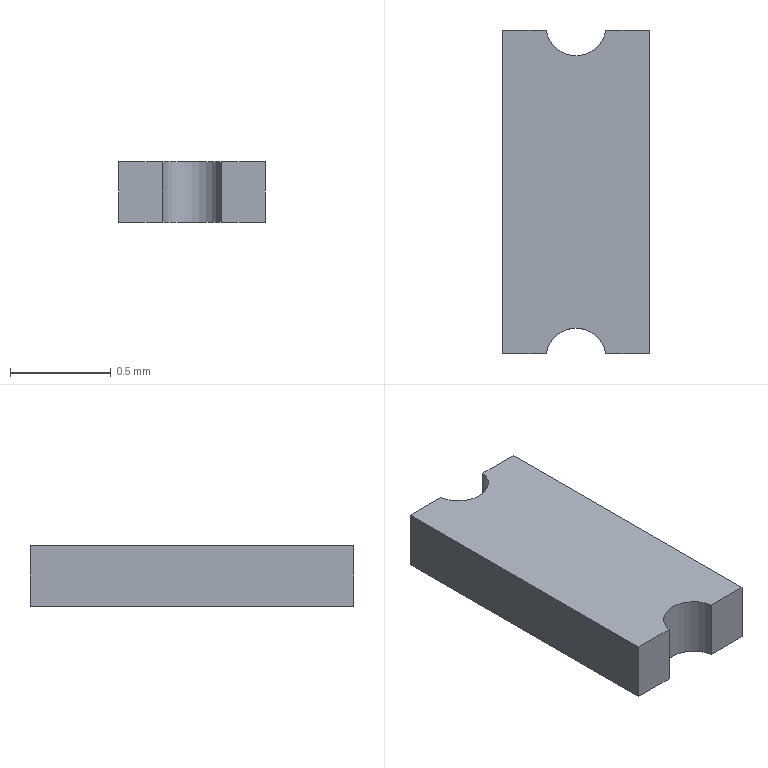Part | STEP file | RJ-USIO-V1_2-220411_160 | 1 solid | 10 faces | box 0.725 x 1.6 x 0.3 mm | volume 0.3313 mm3 | plane 8 | cylinder 2 | commonest cylinder face diameters 0.3 x2
STEP:
#1=CARTESIAN_POINT('',(0.,0.,0.));
#2=DIRECTION('',(0.,0.,1.));
#3=DIRECTION('',(1.,0.,0.));
#4=AXIS2_PLACEMENT_3D('',#1,#2,#3);
#5=CARTESIAN_POINT('',(60.137,66.1,0.3298));
#6=VERTEX_POINT('',#5);
#7=CARTESIAN_POINT('',(60.137,67.7,0.3298));
#8=VERTEX_POINT('',#7);
#9=CARTESIAN_POINT('',(60.137,66.1,0.3298));
#10=DIRECTION('',(-0.000000175,1.,0.));
#11=VECTOR('',#10,1.);
#12=LINE('',#9,#11);
#13=CARTESIAN_POINT('',(60.5,66.9,0.3298));
#14=DIRECTION('',(0.,0.,1.));
#15=DIRECTION('',(-1.,-0.000000175,0.));
#16=AXIS2_PLACEMENT_3D('',#13,#14,#15);
#17=PLANE('',#16);
#18=CARTESIAN_POINT('',(0.3625,0.8));
#19=DIRECTION('',(0.,-1.));
#20=VECTOR('',#19,1.);
#21=LINE('',#18,#20);
#22=(GEOMETRIC_REPRESENTATION_CONTEXT(2)PARAMETRIC_REPRESENTATION_CONTEXT()REPRESENTATION_CONTEXT('',''));
#23=DEFINITIONAL_REPRESENTATION('',(#21),#22);
#24=PCURVE('',#17,#23);
#25=CARTESIAN_POINT('',(60.137,67.7,0.02977));
#26=DIRECTION('',(-1.,-0.000000175,0.));
#27=DIRECTION('',(-0.000000175,1.,0.));
#28=AXIS2_PLACEMENT_3D('',#25,#26,#27);
#29=PLANE('',#28);
#30=CARTESIAN_POINT('',(-1.6,-0.3));
#31=DIRECTION('',(1.,0.));
#32=VECTOR('',#31,1.);
#33=LINE('',#30,#32);
#34=(GEOMETRIC_REPRESENTATION_CONTEXT(2)PARAMETRIC_REPRESENTATION_CONTEXT()REPRESENTATION_CONTEXT('',''));
#35=DEFINITIONAL_REPRESENTATION('',(#33),#34);
#36=PCURVE('',#29,#35);
#37=SURFACE_CURVE('',#12,(#24,#36),.PCURVE_S1.);
#38=EDGE_CURVE('',#6,#8,#37,.T.);
#39=ORIENTED_EDGE('',*,*,#38,.T.);
#40=CARTESIAN_POINT('',(60.352,67.7,0.3298));
#41=VERTEX_POINT('',#40);
#42=CARTESIAN_POINT('',(60.137,67.7,0.3298));
#43=DIRECTION('',(1.,0.000000175,0.));
#44=VECTOR('',#43,1.);
#45=LINE('',#42,#44);
#46=CARTESIAN_POINT('',(0.3625,-0.8));
#47=DIRECTION('',(-1.,0.));
#48=VECTOR('',#47,1.);
#49=LINE('',#46,#48);
#50=(GEOMETRIC_REPRESENTATION_CONTEXT(2)PARAMETRIC_REPRESENTATION_CONTEXT()REPRESENTATION_CONTEXT('',''));
#51=DEFINITIONAL_REPRESENTATION('',(#49),#50);
#52=PCURVE('',#17,#51);
#53=CARTESIAN_POINT('',(60.862,67.7,0.02977));
#54=DIRECTION('',(-0.000000175,1.,0.));
#55=DIRECTION('',(1.,0.000000175,0.));
#56=AXIS2_PLACEMENT_3D('',#53,#54,#55);
#57=PLANE('',#56);
#58=CARTESIAN_POINT('',(-0.725,-0.3));
#59=DIRECTION('',(1.,0.));
#60=VECTOR('',#59,1.);
#61=LINE('',#58,#60);
#62=(GEOMETRIC_REPRESENTATION_CONTEXT(2)PARAMETRIC_REPRESENTATION_CONTEXT()REPRESENTATION_CONTEXT('',''));
#63=DEFINITIONAL_REPRESENTATION('',(#61),#62);
#64=PCURVE('',#57,#63);
#65=SURFACE_CURVE('',#45,(#52,#64),.PCURVE_S1.);
#66=EDGE_CURVE('',#8,#41,#65,.T.);
#67=ORIENTED_EDGE('',*,*,#66,.T.);
#68=CARTESIAN_POINT('',(60.648,67.7,0.3298));
#69=VERTEX_POINT('',#68);
#70=CARTESIAN_POINT('',(60.5,67.725,0.3298));
#71=DIRECTION('',(0.,0.,-1.));
#72=DIRECTION('',(0.986,-0.1667,0.));
#73=AXIS2_PLACEMENT_3D('',#70,#71,#72);
#74=CIRCLE('',#73,0.15);
#75=CARTESIAN_POINT('',(-0.1479,-0.8));
#76=CARTESIAN_POINT('',(-0.1046,-0.5438));
#77=CARTESIAN_POINT('',(0.0956,-0.7094));
#78=CARTESIAN_POINT('',(0.2958,-0.875));
#79=CARTESIAN_POINT('',(0.0523,-0.9656));
#80=CARTESIAN_POINT('',(-0.1912,-1.056));
#81=CARTESIAN_POINT('',(-0.1479,-0.8));
#82=(BOUNDED_CURVE()B_SPLINE_CURVE(2,(#75,#76,#77,#78,#79,#80,#81),.UNSPECIFIED.,.T.,.F.)B_SPLINE_CURVE_WITH_KNOTS((1,2,2,2,2,1),(-2.094,0.,2.094,4.189,6.283,8.378),.UNSPECIFIED.)CURVE()GEOMETRIC_REPRESENTATION_ITEM()RATIONAL_B_SPLINE_CURVE((1.,0.5,1.,0.5,1.,0.5,1.))REPRESENTATION_ITEM(''));
#83=(GEOMETRIC_REPRESENTATION_CONTEXT(2)PARAMETRIC_REPRESENTATION_CONTEXT()REPRESENTATION_CONTEXT('',''));
#84=DEFINITIONAL_REPRESENTATION('',(#82),#83);
#85=PCURVE('',#17,#84);
#86=CARTESIAN_POINT('',(60.5,67.725,-0.2214));
#87=DIRECTION('',(0.,0.,-1.));
#88=DIRECTION('',(1.,0.000000175,0.));
#89=AXIS2_PLACEMENT_3D('',#86,#87,#88);
#90=CYLINDRICAL_SURFACE('',#89,0.15);
#91=CARTESIAN_POINT('',(0.1674,-0.5512));
#92=DIRECTION('',(1.,0.));
#93=VECTOR('',#92,1.);
#94=LINE('',#91,#93);
#95=(GEOMETRIC_REPRESENTATION_CONTEXT(2)PARAMETRIC_REPRESENTATION_CONTEXT()REPRESENTATION_CONTEXT('',''));
#96=DEFINITIONAL_REPRESENTATION('',(#94),#95);
#97=PCURVE('',#90,#96);
#98=SURFACE_CURVE('',#74,(#85,#97),.PCURVE_S1.);
#99=EDGE_CURVE('',#69,#41,#98,.T.);
#100=ORIENTED_EDGE('',*,*,#99,.F.);
#101=CARTESIAN_POINT('',(60.862,67.7,0.3298));
#102=VERTEX_POINT('',#101);
#103=CARTESIAN_POINT('',(60.648,67.7,0.3298));
#104=DIRECTION('',(1.,0.000000175,0.));
#105=VECTOR('',#104,1.);
#106=LINE('',#103,#105);
#107=CARTESIAN_POINT('',(-0.1479,-0.8));
#108=DIRECTION('',(-1.,0.));
#109=VECTOR('',#108,1.);
#110=LINE('',#107,#109);
#111=(GEOMETRIC_REPRESENTATION_CONTEXT(2)PARAMETRIC_REPRESENTATION_CONTEXT()REPRESENTATION_CONTEXT('',''));
#112=DEFINITIONAL_REPRESENTATION('',(#110),#111);
#113=PCURVE('',#17,#112);
#114=CARTESIAN_POINT('',(60.862,67.7,0.02977));
#115=DIRECTION('',(-0.000000175,1.,0.));
#116=DIRECTION('',(1.,0.000000175,0.));
#117=AXIS2_PLACEMENT_3D('',#114,#115,#116);
#118=PLANE('',#117);
#119=CARTESIAN_POINT('',(-0.2146,-0.3));
#120=DIRECTION('',(1.,0.));
#121=VECTOR('',#120,1.);
#122=LINE('',#119,#121);
#123=(GEOMETRIC_REPRESENTATION_CONTEXT(2)PARAMETRIC_REPRESENTATION_CONTEXT()REPRESENTATION_CONTEXT('',''));
#124=DEFINITIONAL_REPRESENTATION('',(#122),#123);
#125=PCURVE('',#118,#124);
#126=SURFACE_CURVE('',#106,(#113,#125),.PCURVE_S1.);
#127=EDGE_CURVE('',#69,#102,#126,.T.);
#128=ORIENTED_EDGE('',*,*,#127,.T.);
#129=CARTESIAN_POINT('',(60.862,66.1,0.3298));
#130=VERTEX_POINT('',#129);
#131=CARTESIAN_POINT('',(60.862,67.7,0.3298));
#132=DIRECTION('',(0.000000175,-1.,0.));
#133=VECTOR('',#132,1.);
#134=LINE('',#131,#133);
#135=CARTESIAN_POINT('',(-0.3625,-0.8));
#136=DIRECTION('',(0.,1.));
#137=VECTOR('',#136,1.);
#138=LINE('',#135,#137);
#139=(GEOMETRIC_REPRESENTATION_CONTEXT(2)PARAMETRIC_REPRESENTATION_CONTEXT()REPRESENTATION_CONTEXT('',''));
#140=DEFINITIONAL_REPRESENTATION('',(#138),#139);
#141=PCURVE('',#17,#140);
#142=CARTESIAN_POINT('',(60.862,66.1,0.02977));
#143=DIRECTION('',(1.,0.000000175,0.));
#144=DIRECTION('',(0.000000175,-1.,0.));
#145=AXIS2_PLACEMENT_3D('',#142,#143,#144);
#146=PLANE('',#145);
#147=CARTESIAN_POINT('',(-1.6,-0.3));
#148=DIRECTION('',(1.,0.));
#149=VECTOR('',#148,1.);
#150=LINE('',#147,#149);
#151=(GEOMETRIC_REPRESENTATION_CONTEXT(2)PARAMETRIC_REPRESENTATION_CONTEXT()REPRESENTATION_CONTEXT('',''));
#152=DEFINITIONAL_REPRESENTATION('',(#150),#151);
#153=PCURVE('',#146,#152);
#154=SURFACE_CURVE('',#134,(#141,#153),.PCURVE_S1.);
#155=EDGE_CURVE('',#102,#130,#154,.T.);
#156=ORIENTED_EDGE('',*,*,#155,.T.);
#157=CARTESIAN_POINT('',(60.648,66.1,0.3298));
#158=VERTEX_POINT('',#157);
#159=CARTESIAN_POINT('',(60.862,66.1,0.3298));
#160=DIRECTION('',(-1.,-0.000000175,0.));
#161=VECTOR('',#160,1.);
#162=LINE('',#159,#161);
#163=CARTESIAN_POINT('',(-0.3625,0.8));
#164=DIRECTION('',(1.,0.));
#165=VECTOR('',#164,1.);
#166=LINE('',#163,#165);
#167=(GEOMETRIC_REPRESENTATION_CONTEXT(2)PARAMETRIC_REPRESENTATION_CONTEXT()REPRESENTATION_CONTEXT('',''));
#168=DEFINITIONAL_REPRESENTATION('',(#166),#167);
#169=PCURVE('',#17,#168);
#170=CARTESIAN_POINT('',(60.862,66.1,0.02977));
#171=DIRECTION('',(0.000000175,-1.,0.));
#172=DIRECTION('',(-1.,-0.000000175,0.));
#173=AXIS2_PLACEMENT_3D('',#170,#171,#172);
#174=PLANE('',#173);
#175=CARTESIAN_POINT('',(0.,-0.3));
#176=DIRECTION('',(1.,0.));
#177=VECTOR('',#176,1.);
#178=LINE('',#175,#177);
#179=(GEOMETRIC_REPRESENTATION_CONTEXT(2)PARAMETRIC_REPRESENTATION_CONTEXT()REPRESENTATION_CONTEXT('',''));
#180=DEFINITIONAL_REPRESENTATION('',(#178),#179);
#181=PCURVE('',#174,#180);
#182=SURFACE_CURVE('',#162,(#169,#181),.PCURVE_S1.);
#183=EDGE_CURVE('',#130,#158,#182,.T.);
#184=ORIENTED_EDGE('',*,*,#183,.T.);
#185=CARTESIAN_POINT('',(60.352,66.1,0.3298));
#186=VERTEX_POINT('',#185);
#187=CARTESIAN_POINT('',(60.5,66.075,0.3298));
#188=DIRECTION('',(0.,0.,-1.));
#189=DIRECTION('',(-0.986,0.1667,0.));
#190=AXIS2_PLACEMENT_3D('',#187,#188,#189);
#191=CIRCLE('',#190,0.15);
#192=CARTESIAN_POINT('',(0.1479,0.8));
#193=CARTESIAN_POINT('',(0.1046,0.5438));
#194=CARTESIAN_POINT('',(-0.0956,0.7094));
#195=CARTESIAN_POINT('',(-0.2958,0.875));
#196=CARTESIAN_POINT('',(-0.0523,0.9656));
#197=CARTESIAN_POINT('',(0.1912,1.056));
#198=CARTESIAN_POINT('',(0.1479,0.8));
#199=(BOUNDED_CURVE()B_SPLINE_CURVE(2,(#192,#193,#194,#195,#196,#197,#198),.UNSPECIFIED.,.T.,.F.)B_SPLINE_CURVE_WITH_KNOTS((1,2,2,2,2,1),(-2.094,0.,2.094,4.189,6.283,8.378),.UNSPECIFIED.)CURVE()GEOMETRIC_REPRESENTATION_ITEM()RATIONAL_B_SPLINE_CURVE((1.,0.5,1.,0.5,1.,0.5,1.))REPRESENTATION_ITEM(''));
#200=(GEOMETRIC_REPRESENTATION_CONTEXT(2)PARAMETRIC_REPRESENTATION_CONTEXT()REPRESENTATION_CONTEXT('',''));
#201=DEFINITIONAL_REPRESENTATION('',(#199),#200);
#202=PCURVE('',#17,#201);
#203=CARTESIAN_POINT('',(60.5,66.075,-0.2214));
#204=DIRECTION('',(0.,0.,1.));
#205=DIRECTION('',(-1.,-0.000000175,0.));
#206=AXIS2_PLACEMENT_3D('',#203,#204,#205);
#207=CYLINDRICAL_SURFACE('',#206,0.15);
#208=CARTESIAN_POINT('',(6.116,0.5512));
#209=DIRECTION('',(-1.,0.));
#210=VECTOR('',#209,1.);
#211=LINE('',#208,#210);
#212=(GEOMETRIC_REPRESENTATION_CONTEXT(2)PARAMETRIC_REPRESENTATION_CONTEXT()REPRESENTATION_CONTEXT('',''));
#213=DEFINITIONAL_REPRESENTATION('',(#211),#212);
#214=PCURVE('',#207,#213);
#215=SURFACE_CURVE('',#191,(#202,#214),.PCURVE_S1.);
#216=EDGE_CURVE('',#186,#158,#215,.T.);
#217=ORIENTED_EDGE('',*,*,#216,.F.);
#218=CARTESIAN_POINT('',(60.352,66.1,0.3298));
#219=DIRECTION('',(-1.,-0.000000175,0.));
#220=VECTOR('',#219,1.);
#221=LINE('',#218,#220);
#222=CARTESIAN_POINT('',(0.1479,0.8));
#223=DIRECTION('',(1.,0.));
#224=VECTOR('',#223,1.);
#225=LINE('',#222,#224);
#226=(GEOMETRIC_REPRESENTATION_CONTEXT(2)PARAMETRIC_REPRESENTATION_CONTEXT()REPRESENTATION_CONTEXT('',''));
#227=DEFINITIONAL_REPRESENTATION('',(#225),#226);
#228=PCURVE('',#17,#227);
#229=CARTESIAN_POINT('',(60.862,66.1,0.02977));
#230=DIRECTION('',(0.000000175,-1.,0.));
#231=DIRECTION('',(-1.,-0.000000175,0.));
#232=AXIS2_PLACEMENT_3D('',#229,#230,#231);
#233=PLANE('',#232);
#234=CARTESIAN_POINT('',(0.5104,-0.3));
#235=DIRECTION('',(1.,0.));
#236=VECTOR('',#235,1.);
#237=LINE('',#234,#236);
#238=(GEOMETRIC_REPRESENTATION_CONTEXT(2)PARAMETRIC_REPRESENTATION_CONTEXT()REPRESENTATION_CONTEXT('',''));
#239=DEFINITIONAL_REPRESENTATION('',(#237),#238);
#240=PCURVE('',#233,#239);
#241=SURFACE_CURVE('',#221,(#228,#240),.PCURVE_S1.);
#242=EDGE_CURVE('',#186,#6,#241,.T.);
#243=ORIENTED_EDGE('',*,*,#242,.T.);
#244=EDGE_LOOP('',(#39,#67,#100,#128,#156,#184,#217,#243));
#245=FACE_BOUND('',#244,.F.);
#246=ADVANCED_FACE('',(#245),#17,.T.);
#247=ORIENTED_EDGE('',*,*,#38,.F.);
#248=CARTESIAN_POINT('',(60.137,66.1,0.02977));
#249=VERTEX_POINT('',#248);
#250=CARTESIAN_POINT('',(60.137,66.1,0.02977));
#251=DIRECTION('',(0.,0.,1.));
#252=VECTOR('',#251,1.);
#253=LINE('',#250,#252);
#254=CARTESIAN_POINT('',(-1.6,0.));
#255=DIRECTION('',(0.,-1.));
#256=VECTOR('',#255,1.);
#257=LINE('',#254,#256);
#258=(GEOMETRIC_REPRESENTATION_CONTEXT(2)PARAMETRIC_REPRESENTATION_CONTEXT()REPRESENTATION_CONTEXT('',''));
#259=DEFINITIONAL_REPRESENTATION('',(#257),#258);
#260=PCURVE('',#29,#259);
#261=CARTESIAN_POINT('',(0.725,0.));
#262=DIRECTION('',(0.,-1.));
#263=VECTOR('',#262,1.);
#264=LINE('',#261,#263);
#265=(GEOMETRIC_REPRESENTATION_CONTEXT(2)PARAMETRIC_REPRESENTATION_CONTEXT()REPRESENTATION_CONTEXT('',''));
#266=DEFINITIONAL_REPRESENTATION('',(#264),#265);
#267=PCURVE('',#233,#266);
#268=SURFACE_CURVE('',#253,(#260,#267),.PCURVE_S1.);
#269=EDGE_CURVE('',#249,#6,#268,.T.);
#270=ORIENTED_EDGE('',*,*,#269,.F.);
#271=CARTESIAN_POINT('',(60.137,67.7,0.02977));
#272=VERTEX_POINT('',#271);
#273=CARTESIAN_POINT('',(60.137,66.1,0.02977));
#274=DIRECTION('',(-0.000000175,1.,0.));
#275=VECTOR('',#274,1.);
#276=LINE('',#273,#275);
#277=CARTESIAN_POINT('',(-1.6,0.));
#278=DIRECTION('',(1.,0.));
#279=VECTOR('',#278,1.);
#280=LINE('',#277,#279);
#281=(GEOMETRIC_REPRESENTATION_CONTEXT(2)PARAMETRIC_REPRESENTATION_CONTEXT()REPRESENTATION_CONTEXT('',''));
#282=DEFINITIONAL_REPRESENTATION('',(#280),#281);
#283=PCURVE('',#29,#282);
#284=CARTESIAN_POINT('',(60.5,66.9,0.02977));
#285=DIRECTION('',(0.,0.,1.));
#286=DIRECTION('',(-1.,-0.000000175,0.));
#287=AXIS2_PLACEMENT_3D('',#284,#285,#286);
#288=PLANE('',#287);
#289=CARTESIAN_POINT('',(0.3625,0.8));
#290=DIRECTION('',(0.,-1.));
#291=VECTOR('',#290,1.);
#292=LINE('',#289,#291);
#293=(GEOMETRIC_REPRESENTATION_CONTEXT(2)PARAMETRIC_REPRESENTATION_CONTEXT()REPRESENTATION_CONTEXT('',''));
#294=DEFINITIONAL_REPRESENTATION('',(#292),#293);
#295=PCURVE('',#288,#294);
#296=SURFACE_CURVE('',#276,(#283,#295),.PCURVE_S1.);
#297=EDGE_CURVE('',#249,#272,#296,.T.);
#298=ORIENTED_EDGE('',*,*,#297,.T.);
#299=CARTESIAN_POINT('',(60.137,67.7,0.02977));
#300=DIRECTION('',(0.,0.,1.));
#301=VECTOR('',#300,1.);
#302=LINE('',#299,#301);
#303=CARTESIAN_POINT('',(0.,0.));
#304=DIRECTION('',(0.,-1.));
#305=VECTOR('',#304,1.);
#306=LINE('',#303,#305);
#307=(GEOMETRIC_REPRESENTATION_CONTEXT(2)PARAMETRIC_REPRESENTATION_CONTEXT()REPRESENTATION_CONTEXT('',''));
#308=DEFINITIONAL_REPRESENTATION('',(#306),#307);
#309=PCURVE('',#29,#308);
#310=CARTESIAN_POINT('',(-0.725,0.));
#311=DIRECTION('',(0.,-1.));
#312=VECTOR('',#311,1.);
#313=LINE('',#310,#312);
#314=(GEOMETRIC_REPRESENTATION_CONTEXT(2)PARAMETRIC_REPRESENTATION_CONTEXT()REPRESENTATION_CONTEXT('',''));
#315=DEFINITIONAL_REPRESENTATION('',(#313),#314);
#316=PCURVE('',#57,#315);
#317=SURFACE_CURVE('',#302,(#309,#316),.PCURVE_S1.);
#318=EDGE_CURVE('',#272,#8,#317,.T.);
#319=ORIENTED_EDGE('',*,*,#318,.T.);
#320=EDGE_LOOP('',(#247,#270,#298,#319));
#321=FACE_BOUND('',#320,.F.);
#322=ADVANCED_FACE('',(#321),#29,.T.);
#323=CARTESIAN_POINT('',(60.352,66.1,0.02977));
#324=VERTEX_POINT('',#323);
#325=CARTESIAN_POINT('',(60.352,66.1,0.3298));
#326=DIRECTION('',(0.,0.,-1.));
#327=VECTOR('',#326,1.);
#328=LINE('',#325,#327);
#329=CARTESIAN_POINT('',(0.5104,-0.3));
#330=DIRECTION('',(0.,1.));
#331=VECTOR('',#330,1.);
#332=LINE('',#329,#331);
#333=(GEOMETRIC_REPRESENTATION_CONTEXT(2)PARAMETRIC_REPRESENTATION_CONTEXT()REPRESENTATION_CONTEXT('',''));
#334=DEFINITIONAL_REPRESENTATION('',(#332),#333);
#335=PCURVE('',#233,#334);
#336=CARTESIAN_POINT('',(6.116,0.5512));
#337=DIRECTION('',(0.,-1.));
#338=VECTOR('',#337,1.);
#339=LINE('',#336,#338);
#340=(GEOMETRIC_REPRESENTATION_CONTEXT(2)PARAMETRIC_REPRESENTATION_CONTEXT()REPRESENTATION_CONTEXT('',''));
#341=DEFINITIONAL_REPRESENTATION('',(#339),#340);
#342=PCURVE('',#207,#341);
#343=SURFACE_CURVE('',#328,(#335,#342),.PCURVE_S1.);
#344=EDGE_CURVE('',#186,#324,#343,.T.);
#345=ORIENTED_EDGE('',*,*,#344,.T.);
#346=CARTESIAN_POINT('',(60.352,66.1,0.02977));
#347=DIRECTION('',(-1.,-0.000000175,0.));
#348=VECTOR('',#347,1.);
#349=LINE('',#346,#348);
#350=CARTESIAN_POINT('',(0.5104,0.));
#351=DIRECTION('',(1.,0.));
#352=VECTOR('',#351,1.);
#353=LINE('',#350,#352);
#354=(GEOMETRIC_REPRESENTATION_CONTEXT(2)PARAMETRIC_REPRESENTATION_CONTEXT()REPRESENTATION_CONTEXT('',''));
#355=DEFINITIONAL_REPRESENTATION('',(#353),#354);
#356=PCURVE('',#233,#355);
#357=CARTESIAN_POINT('',(0.1479,0.8));
#358=DIRECTION('',(1.,0.));
#359=VECTOR('',#358,1.);
#360=LINE('',#357,#359);
#361=(GEOMETRIC_REPRESENTATION_CONTEXT(2)PARAMETRIC_REPRESENTATION_CONTEXT()REPRESENTATION_CONTEXT('',''));
#362=DEFINITIONAL_REPRESENTATION('',(#360),#361);
#363=PCURVE('',#288,#362);
#364=SURFACE_CURVE('',#349,(#356,#363),.PCURVE_S1.);
#365=EDGE_CURVE('',#324,#249,#364,.T.);
#366=ORIENTED_EDGE('',*,*,#365,.T.);
#367=ORIENTED_EDGE('',*,*,#269,.T.);
#368=ORIENTED_EDGE('',*,*,#242,.F.);
#369=EDGE_LOOP('',(#345,#366,#367,#368));
#370=FACE_BOUND('',#369,.F.);
#371=ADVANCED_FACE('',(#370),#233,.T.);
#372=CARTESIAN_POINT('',(60.648,66.1,0.02977));
#373=VERTEX_POINT('',#372);
#374=CARTESIAN_POINT('',(60.5,66.075,0.02977));
#375=DIRECTION('',(0.,0.,1.));
#376=DIRECTION('',(0.986,0.1667,0.));
#377=AXIS2_PLACEMENT_3D('',#374,#375,#376);
#378=CIRCLE('',#377,0.15);
#379=CARTESIAN_POINT('',(3.309,0.2512));
#380=DIRECTION('',(1.,0.));
#381=VECTOR('',#380,1.);
#382=LINE('',#379,#381);
#383=(GEOMETRIC_REPRESENTATION_CONTEXT(2)PARAMETRIC_REPRESENTATION_CONTEXT()REPRESENTATION_CONTEXT('',''));
#384=DEFINITIONAL_REPRESENTATION('',(#382),#383);
#385=PCURVE('',#207,#384);
#386=CARTESIAN_POINT('',(0.,0.825));
#387=DIRECTION('',(-0.986,-0.1667));
#388=AXIS2_PLACEMENT_2D('',#386,#387);
#389=CIRCLE('',#388,0.15);
#390=(GEOMETRIC_REPRESENTATION_CONTEXT(2)PARAMETRIC_REPRESENTATION_CONTEXT()REPRESENTATION_CONTEXT('',''));
#391=DEFINITIONAL_REPRESENTATION('',(#389),#390);
#392=PCURVE('',#288,#391);
#393=SURFACE_CURVE('',#378,(#385,#392),.PCURVE_S1.);
#394=EDGE_CURVE('',#373,#324,#393,.T.);
#395=ORIENTED_EDGE('',*,*,#394,.T.);
#396=ORIENTED_EDGE('',*,*,#344,.F.);
#397=ORIENTED_EDGE('',*,*,#216,.T.);
#398=CARTESIAN_POINT('',(60.648,66.1,0.02977));
#399=DIRECTION('',(0.,0.,1.));
#400=VECTOR('',#399,1.);
#401=LINE('',#398,#400);
#402=CARTESIAN_POINT('',(3.309,0.2512));
#403=DIRECTION('',(0.,1.));
#404=VECTOR('',#403,1.);
#405=LINE('',#402,#404);
#406=(GEOMETRIC_REPRESENTATION_CONTEXT(2)PARAMETRIC_REPRESENTATION_CONTEXT()REPRESENTATION_CONTEXT('',''));
#407=DEFINITIONAL_REPRESENTATION('',(#405),#406);
#408=PCURVE('',#207,#407);
#409=CARTESIAN_POINT('',(0.2146,0.));
#410=DIRECTION('',(0.,-1.));
#411=VECTOR('',#410,1.);
#412=LINE('',#409,#411);
#413=(GEOMETRIC_REPRESENTATION_CONTEXT(2)PARAMETRIC_REPRESENTATION_CONTEXT()REPRESENTATION_CONTEXT('',''));
#414=DEFINITIONAL_REPRESENTATION('',(#412),#413);
#415=PCURVE('',#174,#414);
#416=SURFACE_CURVE('',#401,(#408,#415),.PCURVE_S1.);
#417=EDGE_CURVE('',#373,#158,#416,.T.);
#418=ORIENTED_EDGE('',*,*,#417,.F.);
#419=EDGE_LOOP('',(#395,#396,#397,#418));
#420=FACE_BOUND('',#419,.F.);
#421=ADVANCED_FACE('',(#420),#207,.F.);
#422=CARTESIAN_POINT('',(60.352,67.7,0.02977));
#423=VERTEX_POINT('',#422);
#424=CARTESIAN_POINT('',(60.648,67.7,0.02977));
#425=VERTEX_POINT('',#424);
#426=CARTESIAN_POINT('',(60.5,67.725,0.02977));
#427=DIRECTION('',(0.,0.,1.));
#428=DIRECTION('',(-0.986,-0.1667,0.));
#429=AXIS2_PLACEMENT_3D('',#426,#427,#428);
#430=CIRCLE('',#429,0.15);
#431=CARTESIAN_POINT('',(0.,-0.825));
#432=DIRECTION('',(0.986,0.1667));
#433=AXIS2_PLACEMENT_2D('',#431,#432);
#434=CIRCLE('',#433,0.15);
#435=(GEOMETRIC_REPRESENTATION_CONTEXT(2)PARAMETRIC_REPRESENTATION_CONTEXT()REPRESENTATION_CONTEXT('',''));
#436=DEFINITIONAL_REPRESENTATION('',(#434),#435);
#437=PCURVE('',#288,#436);
#438=CARTESIAN_POINT('',(2.974,-0.2512));
#439=DIRECTION('',(-1.,0.));
#440=VECTOR('',#439,1.);
#441=LINE('',#438,#440);
#442=(GEOMETRIC_REPRESENTATION_CONTEXT(2)PARAMETRIC_REPRESENTATION_CONTEXT()REPRESENTATION_CONTEXT('',''));
#443=DEFINITIONAL_REPRESENTATION('',(#441),#442);
#444=PCURVE('',#90,#443);
#445=SURFACE_CURVE('',#430,(#437,#444),.PCURVE_S1.);
#446=EDGE_CURVE('',#423,#425,#445,.T.);
#447=ORIENTED_EDGE('',*,*,#446,.F.);
#448=CARTESIAN_POINT('',(60.137,67.7,0.02977));
#449=DIRECTION('',(1.,0.000000175,0.));
#450=VECTOR('',#449,1.);
#451=LINE('',#448,#450);
#452=CARTESIAN_POINT('',(0.3625,-0.8));
#453=DIRECTION('',(-1.,0.));
#454=VECTOR('',#453,1.);
#455=LINE('',#452,#454);
#456=(GEOMETRIC_REPRESENTATION_CONTEXT(2)PARAMETRIC_REPRESENTATION_CONTEXT()REPRESENTATION_CONTEXT('',''));
#457=DEFINITIONAL_REPRESENTATION('',(#455),#456);
#458=PCURVE('',#288,#457);
#459=CARTESIAN_POINT('',(-0.725,0.));
#460=DIRECTION('',(1.,0.));
#461=VECTOR('',#460,1.);
#462=LINE('',#459,#461);
#463=(GEOMETRIC_REPRESENTATION_CONTEXT(2)PARAMETRIC_REPRESENTATION_CONTEXT()REPRESENTATION_CONTEXT('',''));
#464=DEFINITIONAL_REPRESENTATION('',(#462),#463);
#465=PCURVE('',#57,#464);
#466=SURFACE_CURVE('',#451,(#458,#465),.PCURVE_S1.);
#467=EDGE_CURVE('',#272,#423,#466,.T.);
#468=ORIENTED_EDGE('',*,*,#467,.F.);
#469=ORIENTED_EDGE('',*,*,#297,.F.);
#470=ORIENTED_EDGE('',*,*,#365,.F.);
#471=ORIENTED_EDGE('',*,*,#394,.F.);
#472=CARTESIAN_POINT('',(60.862,66.1,0.02977));
#473=VERTEX_POINT('',#472);
#474=CARTESIAN_POINT('',(60.862,66.1,0.02977));
#475=DIRECTION('',(-1.,-0.000000175,0.));
#476=VECTOR('',#475,1.);
#477=LINE('',#474,#476);
#478=CARTESIAN_POINT('',(-0.3625,0.8));
#479=DIRECTION('',(1.,0.));
#480=VECTOR('',#479,1.);
#481=LINE('',#478,#480);
#482=(GEOMETRIC_REPRESENTATION_CONTEXT(2)PARAMETRIC_REPRESENTATION_CONTEXT()REPRESENTATION_CONTEXT('',''));
#483=DEFINITIONAL_REPRESENTATION('',(#481),#482);
#484=PCURVE('',#288,#483);
#485=CARTESIAN_POINT('',(0.,0.));
#486=DIRECTION('',(1.,0.));
#487=VECTOR('',#486,1.);
#488=LINE('',#485,#487);
#489=(GEOMETRIC_REPRESENTATION_CONTEXT(2)PARAMETRIC_REPRESENTATION_CONTEXT()REPRESENTATION_CONTEXT('',''));
#490=DEFINITIONAL_REPRESENTATION('',(#488),#489);
#491=PCURVE('',#174,#490);
#492=SURFACE_CURVE('',#477,(#484,#491),.PCURVE_S1.);
#493=EDGE_CURVE('',#473,#373,#492,.T.);
#494=ORIENTED_EDGE('',*,*,#493,.F.);
#495=CARTESIAN_POINT('',(60.862,67.7,0.02977));
#496=VERTEX_POINT('',#495);
#497=CARTESIAN_POINT('',(60.862,67.7,0.02977));
#498=DIRECTION('',(0.000000175,-1.,0.));
#499=VECTOR('',#498,1.);
#500=LINE('',#497,#499);
#501=CARTESIAN_POINT('',(-0.3625,-0.8));
#502=DIRECTION('',(0.,1.));
#503=VECTOR('',#502,1.);
#504=LINE('',#501,#503);
#505=(GEOMETRIC_REPRESENTATION_CONTEXT(2)PARAMETRIC_REPRESENTATION_CONTEXT()REPRESENTATION_CONTEXT('',''));
#506=DEFINITIONAL_REPRESENTATION('',(#504),#505);
#507=PCURVE('',#288,#506);
#508=CARTESIAN_POINT('',(-1.6,0.));
#509=DIRECTION('',(1.,0.));
#510=VECTOR('',#509,1.);
#511=LINE('',#508,#510);
#512=(GEOMETRIC_REPRESENTATION_CONTEXT(2)PARAMETRIC_REPRESENTATION_CONTEXT()REPRESENTATION_CONTEXT('',''));
#513=DEFINITIONAL_REPRESENTATION('',(#511),#512);
#514=PCURVE('',#146,#513);
#515=SURFACE_CURVE('',#500,(#507,#514),.PCURVE_S1.);
#516=EDGE_CURVE('',#496,#473,#515,.T.);
#517=ORIENTED_EDGE('',*,*,#516,.F.);
#518=CARTESIAN_POINT('',(60.648,67.7,0.02977));
#519=DIRECTION('',(1.,0.000000175,0.));
#520=VECTOR('',#519,1.);
#521=LINE('',#518,#520);
#522=CARTESIAN_POINT('',(-0.1479,-0.8));
#523=DIRECTION('',(-1.,0.));
#524=VECTOR('',#523,1.);
#525=LINE('',#522,#524);
#526=(GEOMETRIC_REPRESENTATION_CONTEXT(2)PARAMETRIC_REPRESENTATION_CONTEXT()REPRESENTATION_CONTEXT('',''));
#527=DEFINITIONAL_REPRESENTATION('',(#525),#526);
#528=PCURVE('',#288,#527);
#529=CARTESIAN_POINT('',(-0.2146,0.));
#530=DIRECTION('',(1.,0.));
#531=VECTOR('',#530,1.);
#532=LINE('',#529,#531);
#533=(GEOMETRIC_REPRESENTATION_CONTEXT(2)PARAMETRIC_REPRESENTATION_CONTEXT()REPRESENTATION_CONTEXT('',''));
#534=DEFINITIONAL_REPRESENTATION('',(#532),#533);
#535=PCURVE('',#118,#534);
#536=SURFACE_CURVE('',#521,(#528,#535),.PCURVE_S1.);
#537=EDGE_CURVE('',#425,#496,#536,.T.);
#538=ORIENTED_EDGE('',*,*,#537,.F.);
#539=EDGE_LOOP('',(#447,#468,#469,#470,#471,#494,#517,#538));
#540=FACE_BOUND('',#539,.F.);
#541=ADVANCED_FACE('',(#540),#288,.F.);
#542=CARTESIAN_POINT('',(60.352,67.7,0.02977));
#543=DIRECTION('',(0.,0.,1.));
#544=VECTOR('',#543,1.);
#545=LINE('',#542,#544);
#546=CARTESIAN_POINT('',(2.974,-0.2512));
#547=DIRECTION('',(0.,-1.));
#548=VECTOR('',#547,1.);
#549=LINE('',#546,#548);
#550=(GEOMETRIC_REPRESENTATION_CONTEXT(2)PARAMETRIC_REPRESENTATION_CONTEXT()REPRESENTATION_CONTEXT('',''));
#551=DEFINITIONAL_REPRESENTATION('',(#549),#550);
#552=PCURVE('',#90,#551);
#553=CARTESIAN_POINT('',(-0.5104,0.));
#554=DIRECTION('',(0.,-1.));
#555=VECTOR('',#554,1.);
#556=LINE('',#553,#555);
#557=(GEOMETRIC_REPRESENTATION_CONTEXT(2)PARAMETRIC_REPRESENTATION_CONTEXT()REPRESENTATION_CONTEXT('',''));
#558=DEFINITIONAL_REPRESENTATION('',(#556),#557);
#559=PCURVE('',#57,#558);
#560=SURFACE_CURVE('',#545,(#552,#559),.PCURVE_S1.);
#561=EDGE_CURVE('',#423,#41,#560,.T.);
#562=ORIENTED_EDGE('',*,*,#561,.F.);
#563=ORIENTED_EDGE('',*,*,#446,.T.);
#564=CARTESIAN_POINT('',(60.648,67.7,0.3298));
#565=DIRECTION('',(0.,0.,-1.));
#566=VECTOR('',#565,1.);
#567=LINE('',#564,#566);
#568=CARTESIAN_POINT('',(0.1674,-0.5512));
#569=DIRECTION('',(0.,1.));
#570=VECTOR('',#569,1.);
#571=LINE('',#568,#570);
#572=(GEOMETRIC_REPRESENTATION_CONTEXT(2)PARAMETRIC_REPRESENTATION_CONTEXT()REPRESENTATION_CONTEXT('',''));
#573=DEFINITIONAL_REPRESENTATION('',(#571),#572);
#574=PCURVE('',#90,#573);
#575=CARTESIAN_POINT('',(-0.2146,-0.3));
#576=DIRECTION('',(0.,1.));
#577=VECTOR('',#576,1.);
#578=LINE('',#575,#577);
#579=(GEOMETRIC_REPRESENTATION_CONTEXT(2)PARAMETRIC_REPRESENTATION_CONTEXT()REPRESENTATION_CONTEXT('',''));
#580=DEFINITIONAL_REPRESENTATION('',(#578),#579);
#581=PCURVE('',#118,#580);
#582=SURFACE_CURVE('',#567,(#574,#581),.PCURVE_S1.);
#583=EDGE_CURVE('',#69,#425,#582,.T.);
#584=ORIENTED_EDGE('',*,*,#583,.F.);
#585=ORIENTED_EDGE('',*,*,#99,.T.);
#586=EDGE_LOOP('',(#562,#563,#584,#585));
#587=FACE_BOUND('',#586,.F.);
#588=ADVANCED_FACE('',(#587),#90,.F.);
#589=ORIENTED_EDGE('',*,*,#561,.T.);
#590=ORIENTED_EDGE('',*,*,#66,.F.);
#591=ORIENTED_EDGE('',*,*,#318,.F.);
#592=ORIENTED_EDGE('',*,*,#467,.T.);
#593=EDGE_LOOP('',(#589,#590,#591,#592));
#594=FACE_BOUND('',#593,.F.);
#595=ADVANCED_FACE('',(#594),#57,.T.);
#596=ORIENTED_EDGE('',*,*,#583,.T.);
#597=ORIENTED_EDGE('',*,*,#537,.T.);
#598=CARTESIAN_POINT('',(60.862,67.7,0.02977));
#599=DIRECTION('',(0.,0.,1.));
#600=VECTOR('',#599,1.);
#601=LINE('',#598,#600);
#602=CARTESIAN_POINT('',(0.,0.));
#603=DIRECTION('',(0.,-1.));
#604=VECTOR('',#603,1.);
#605=LINE('',#602,#604);
#606=(GEOMETRIC_REPRESENTATION_CONTEXT(2)PARAMETRIC_REPRESENTATION_CONTEXT()REPRESENTATION_CONTEXT('',''));
#607=DEFINITIONAL_REPRESENTATION('',(#605),#606);
#608=PCURVE('',#118,#607);
#609=CARTESIAN_POINT('',(-1.6,0.));
#610=DIRECTION('',(0.,-1.));
#611=VECTOR('',#610,1.);
#612=LINE('',#609,#611);
#613=(GEOMETRIC_REPRESENTATION_CONTEXT(2)PARAMETRIC_REPRESENTATION_CONTEXT()REPRESENTATION_CONTEXT('',''));
#614=DEFINITIONAL_REPRESENTATION('',(#612),#613);
#615=PCURVE('',#146,#614);
#616=SURFACE_CURVE('',#601,(#608,#615),.PCURVE_S1.);
#617=EDGE_CURVE('',#496,#102,#616,.T.);
#618=ORIENTED_EDGE('',*,*,#617,.T.);
#619=ORIENTED_EDGE('',*,*,#127,.F.);
#620=EDGE_LOOP('',(#596,#597,#618,#619));
#621=FACE_BOUND('',#620,.F.);
#622=ADVANCED_FACE('',(#621),#118,.T.);
#623=ORIENTED_EDGE('',*,*,#516,.T.);
#624=CARTESIAN_POINT('',(60.862,66.1,0.02977));
#625=DIRECTION('',(0.,0.,1.));
#626=VECTOR('',#625,1.);
#627=LINE('',#624,#626);
#628=CARTESIAN_POINT('',(0.,0.));
#629=DIRECTION('',(0.,-1.));
#630=VECTOR('',#629,1.);
#631=LINE('',#628,#630);
#632=(GEOMETRIC_REPRESENTATION_CONTEXT(2)PARAMETRIC_REPRESENTATION_CONTEXT()REPRESENTATION_CONTEXT('',''));
#633=DEFINITIONAL_REPRESENTATION('',(#631),#632);
#634=PCURVE('',#146,#633);
#635=CARTESIAN_POINT('',(0.,0.));
#636=DIRECTION('',(0.,-1.));
#637=VECTOR('',#636,1.);
#638=LINE('',#635,#637);
#639=(GEOMETRIC_REPRESENTATION_CONTEXT(2)PARAMETRIC_REPRESENTATION_CONTEXT()REPRESENTATION_CONTEXT('',''));
#640=DEFINITIONAL_REPRESENTATION('',(#638),#639);
#641=PCURVE('',#174,#640);
#642=SURFACE_CURVE('',#627,(#634,#641),.PCURVE_S1.);
#643=EDGE_CURVE('',#473,#130,#642,.T.);
#644=ORIENTED_EDGE('',*,*,#643,.T.);
#645=ORIENTED_EDGE('',*,*,#155,.F.);
#646=ORIENTED_EDGE('',*,*,#617,.F.);
#647=EDGE_LOOP('',(#623,#644,#645,#646));
#648=FACE_BOUND('',#647,.F.);
#649=ADVANCED_FACE('',(#648),#146,.T.);
#650=ORIENTED_EDGE('',*,*,#417,.T.);
#651=ORIENTED_EDGE('',*,*,#183,.F.);
#652=ORIENTED_EDGE('',*,*,#643,.F.);
#653=ORIENTED_EDGE('',*,*,#493,.T.);
#654=EDGE_LOOP('',(#650,#651,#652,#653));
#655=FACE_BOUND('',#654,.F.);
#656=ADVANCED_FACE('',(#655),#174,.T.);
#657=CLOSED_SHELL('',(#246,#322,#371,#421,#541,#588,#595,#622,#649,#656));
#658=MANIFOLD_SOLID_BREP('',#657);
#659=(LENGTH_UNIT()NAMED_UNIT(*)SI_UNIT(.MILLI.,.METRE.));
#660=UNCERTAINTY_MEASURE_WITH_UNIT(LENGTH_MEASURE(0.0000001),#659,'','');
#661=(NAMED_UNIT(*)PLANE_ANGLE_UNIT()SI_UNIT($,.RADIAN.));
#662=(NAMED_UNIT(*)SI_UNIT($,.STERADIAN.)SOLID_ANGLE_UNIT());
#663=(GEOMETRIC_REPRESENTATION_CONTEXT(3)GLOBAL_UNCERTAINTY_ASSIGNED_CONTEXT((#660))GLOBAL_UNIT_ASSIGNED_CONTEXT((#659,#661,#662))REPRESENTATION_CONTEXT('',''));
#664=ADVANCED_BREP_SHAPE_REPRESENTATION('',(#4,#658),#663);